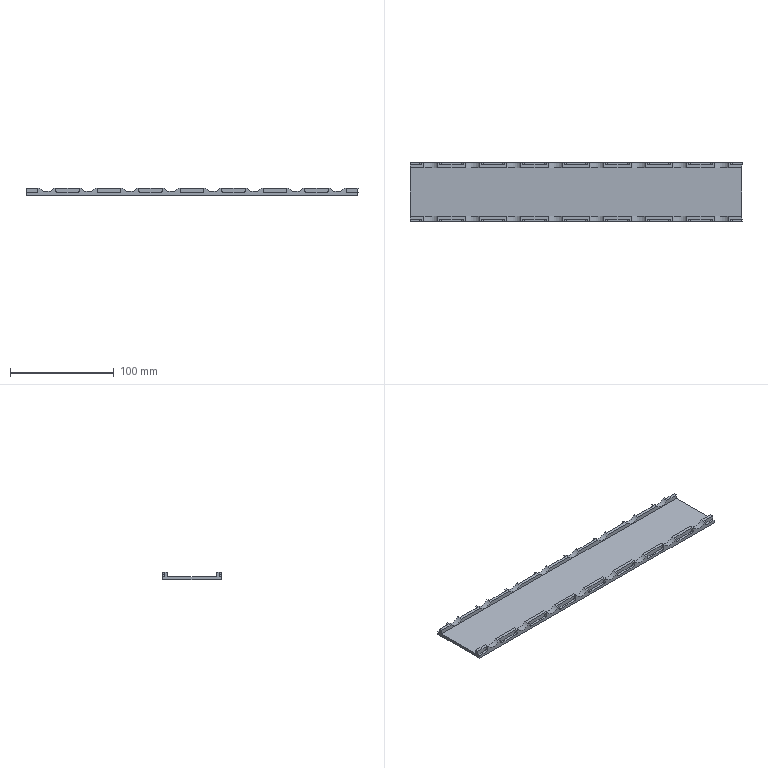CAM job | Mastercam | 3-axis milling, 5-axis milling
Tools:
tool_number,name,type,diameter_mm,corner_radius_mm,flutes,flute_length_mm,overall_length_mm,shoulder_length_mm,holder_diameter_mm,length_offset,diameter_offset,default_rpm,default_feed_mm_min,default_plunge_mm_min,coolant
1,8 Roughing cutter,end mill,8,0,4,25,30,25,50,1,1,6500,2000,2000,COOL_OFF
2,8 Finish cutter,end mill,8,0,4,25,30,25,50,2,2,5500,800,2000,COOL_OFF
3,4 Roughing cutter,end mill,4,0,4,25,25,25,50,3,3,6500,600,2000,COOL_OFF
4,4 Finish cutter,end mill,4,0,4,25,25,25,50,4,4,5500,600,2000,COOL_OFF
5,2 Ball Mill / Bull Nose Mill,ball end mill,2,1,4,20,20,20,50,5,5,6000,720,600,COOL_OFF
Operations:
seq,operation,operation_type,tool_number,tool_name,tool_diameter_mm,spindle_rpm,feed_mm_min,plunge_mm_min,retract_mm_min,cycle_time_s,wcs,posted,nc_file
1,Contour (Ramp) - [WCS: Top] - [Tplane: Top],Contour,1,8 Roughing cutter,8,6500,2000,2000,5000,337.648,Top,yes,.nc
2,Pocket (Standard) - [WCS: Top] - [Tplane: Top],Pocket,1,8 Roughing cutter,8,6500,2000,2000,5000,517.094,Top,yes,.nc
3,Contour (2D) - [WCS: Top] - [Tplane: Top],Contour,1,8 Roughing cutter,8,5000,600,2000,1200,68.074,Top,yes,.nc
4,Pocket (Standard) - [WCS: Top] - [Tplane: Top],Pocket,2,8 Finish cutter,8,6500,1000,2000,5000,208.873,Top,yes,.nc
5,Contour (2D) - [WCS: Top] - [Tplane: Top],Contour,1,8 Roughing cutter,8,5000,600,2000,1200,68.076,Top,yes,.nc
6,Contour (Ramp) - [WCS: Top] - [Tplane: Plane],Contour,1,8 Roughing cutter,8,5000,1000,2000,1200,243.538,Top,yes,.nc
7,Contour (2D) - [WCS: Top] - [Tplane: Plane],Contour,2,8 Finish cutter,8,5000,600,2000,1200,25.67,Top,yes,.nc
8,Contour (Ramp) - [WCS: Top] - [Tplane: Plane],Contour,3,4 Roughing cutter,4,6500,600,2000,5000,435.645,Top,yes,.nc
9,Contour (2D) - [WCS: Top] - [Tplane: Plane],Contour,4,4 Finish cutter,4,6500,600,2000,5000,58.575,Top,yes,.nc
10,Contour (Ramp) - [WCS: Top] - [Tplane: Plane-1],Contour,1,8 Roughing cutter,8,5000,1000,2000,1200,243.538,Top,yes,.nc
11,Contour (2D) - [WCS: Top] - [Tplane: Plane-1],Contour,2,8 Finish cutter,8,5000,600,2000,1200,25.67,Top,yes,.nc
12,Contour (Ramp) - [WCS: Top] - [Tplane: Plane-1],Contour,3,4 Roughing cutter,4,6500,600,2000,5000,435.645,Top,yes,.nc
13,Contour (2D) - [WCS: Top] - [Tplane: Plane-1],Contour,4,4 Finish cutter,4,6500,600,2000,5000,58.575,Top,yes,.nc
14,Deburr 5-axis - [WCS: Top] - [Tplane: Top],459,5,2 Ball Mill / Bull Nose Mill,2,6000,1000,2000,1200,87.342,Top,yes,.nc
15,Contour (2D) - [WCS: Top] - [Tplane: Top],Contour,2,8 Finish cutter,8,6500,600,2000,5000,80.285,Top,yes,.nc